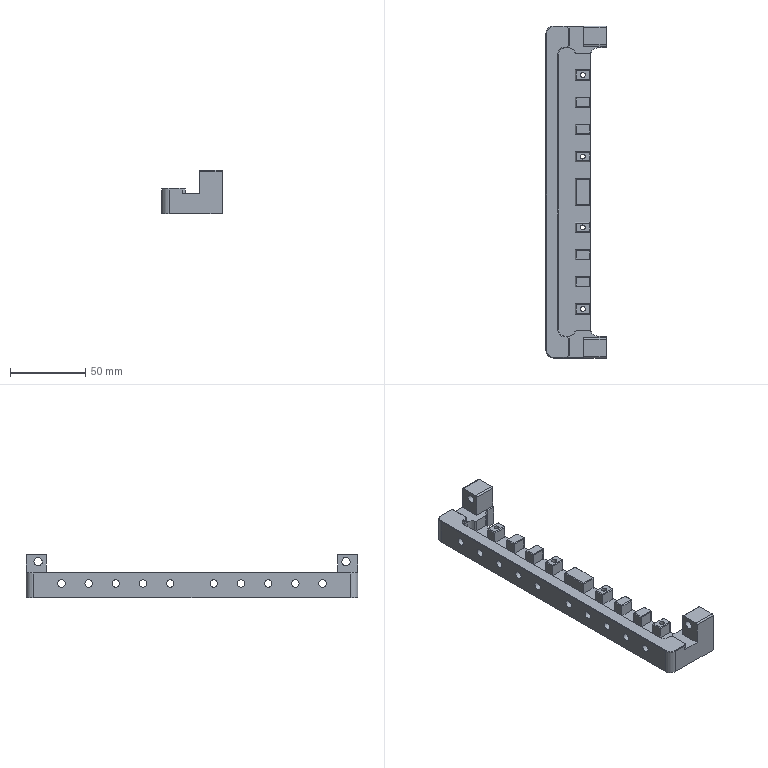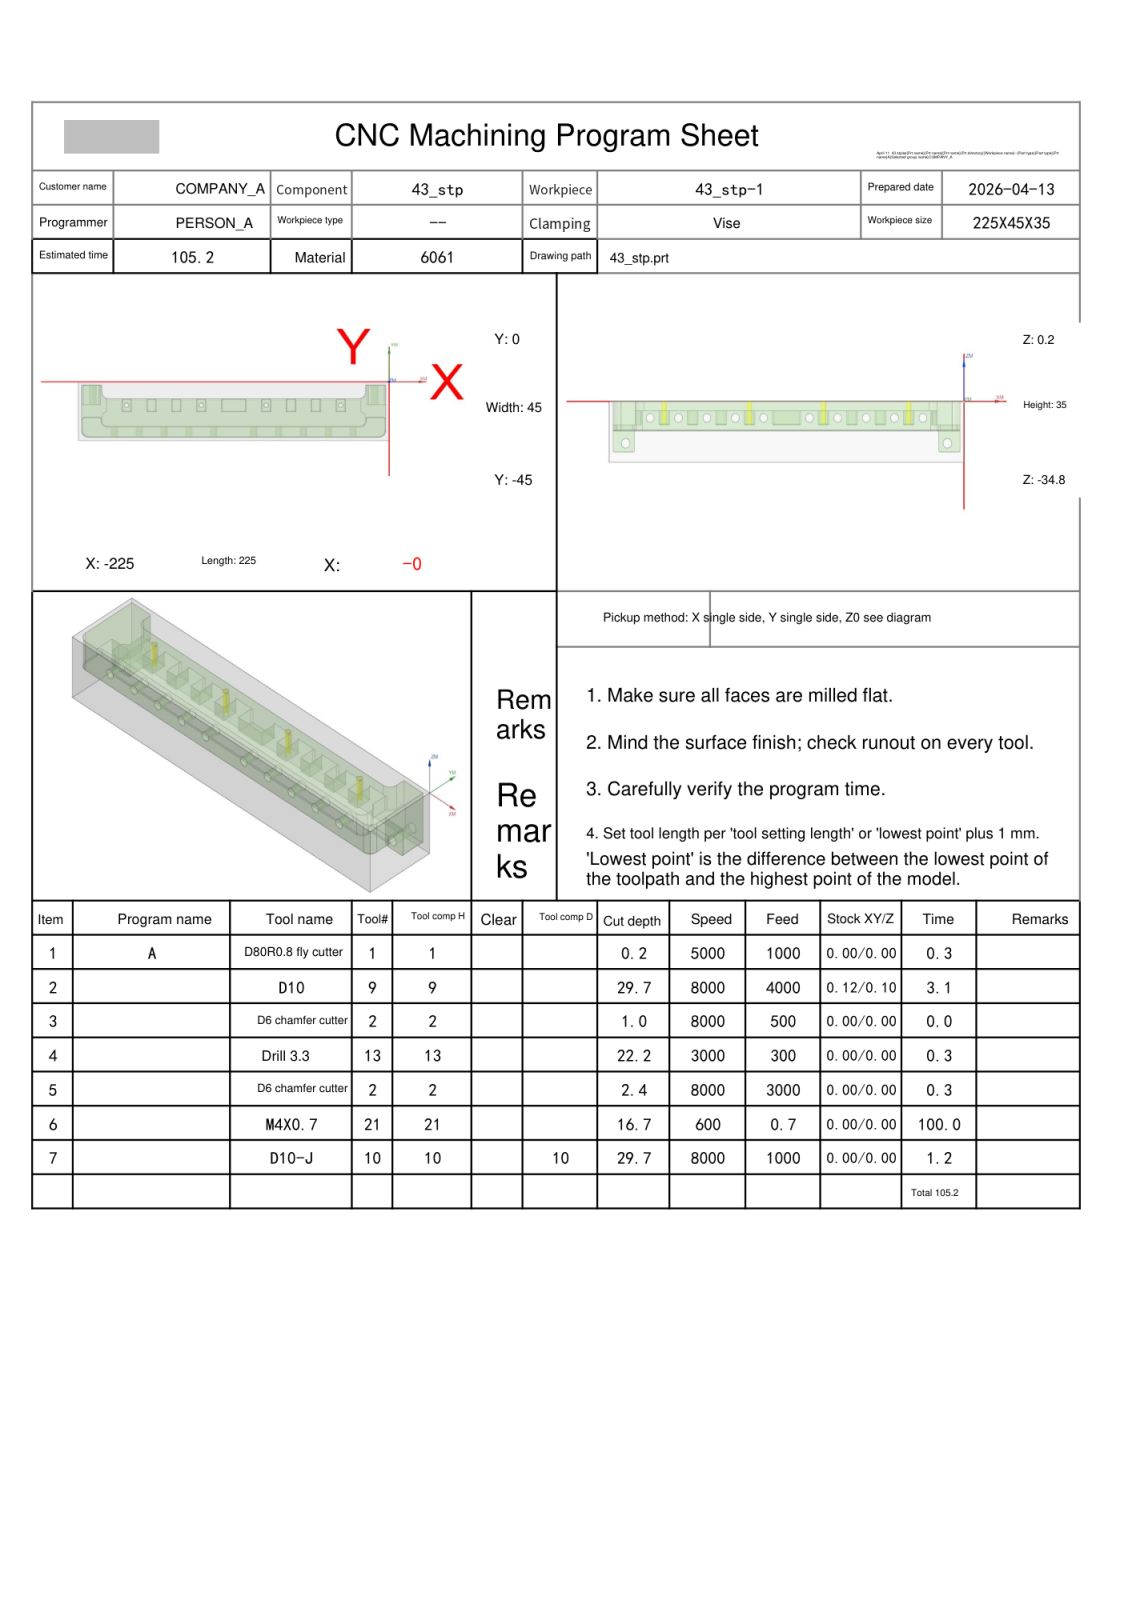NC program | NX | posted by the shop | part box 40 x 220 x 29 mm
Whole program:
%
O0001
(Machine time: 200.90 MIN)
(===Total Tool:6===)
(T1=D80R0.8 fly cutter D=80.  R=0.8  D-  H01 Z=0.    )
(T9=D10     D=10.  R=0.   D-  H09 Z=-29.5 )
(T2=D6 chamfer cutter   D=6.   R=0.   D-  H02 Z=-2.2  )
(T13=drill 3.3  D=3.3  DR_a=118 D-  H13 Z=-22.  )
(T21=M4X0.7 D=3.3  DR_a=180 D-  H21 Z=-16.5 )
(T10=D10-J  D=10.  R=0.   D10 H10 Z=-29.5 )
G80 G90 G17 G49 G40
G91 G28 Z0
M01
N1 T01 M06
(D80R0.8 fly cutter  D=80. R=0.8 H=01 ce=0.00 di=0.00)
G00 G90 G54 X-267.5 Y-22.5 M03 S5000
G43 H01 Z20.
M08
Z2.
G01 Z0.0 F1000.
X-262.5
X37.5
X42.5
Z2.
G00 Z20.
G91 G28 Z0.0
M05
M09
G91 G28 Z0.0
M01
N2 T09 M06
(D10  D=10. R=0. H=09 ce=0.12 di=0.10)
G00 G90 G54 X-223.344 Y10.981 M03 S8000
G43 H09 Z20.
M08
Z-12.75
G01 X-223.325 Y10.882 Z-13.375 F4000.
X-223.306 Y10.784 Z-13.622
X-223.288 Y10.686 Z-13.804
X-223.269 Y10.588 Z-13.95
X-223.25 Y10.489 Z-14.073
X-223.232 Y10.391 Z-14.178
X-223.213 Y10.293 Z-14.27
X-223.194 Y10.195 Z-14.35
X-223.176 Y10.096 Z-14.42
X-223.157 Y9.998 Z-14.482
X-223.138 Y9.9 Z-14.536
X-223.12 Y9.802 Z-14.583
X-223.101 Y9.703 Z-14.624
X-223.082 Y9.605 Z-14.658
X-223.064 Y9.507 Z-14.686
X-223.045 Y9.409 Z-14.71
X-223.026 Y9.311 Z-14.727
X-223.008 Y9.212 Z-14.74
X-222.989 Y9.114 Z-14.747
X-222.97 Y9.016 Z-14.75
X-222.569 Y6.902
G03 X-222.31 Y6.55 I.505 J.101
X-218.496 Y5.912 I4.013 J12.27
X-208.326 Y5.731 I10.17 J285.705
X-205.002 Y5.75 I0.0 J285.885
G01 X-1.882 Y5.733
G02 X4.2 Y1.629 I-.118 J-6.733
X5.522 Y-4.19 I-15.384 J-6.557
X5.77 Y-13.731 I-184.09 J-9.541
X5.749 Y-16.505 I-184.337 J0.0
G01 X5.724 Y-43.28
G02 X1.627 Y-49.201 I-6.717 J.27
X-4.033 Y-50.51 I-6.479 J15.125
X-12.653 Y-50.761 I-8.62 J147.776
X-14.667 Y-50.747 I0.0 J148.027
G01 X-223.127 Y-50.733
G02 X-229.068 Y-46.861 I.104 J6.655
X-230.511 Y-40.908 I14.588 J6.685
X-230.754 Y-32.801 I135.158 J8.107
X-230.745 Y-31.313 I135.401 J0.0
G01 X-230.732 Y-1.86
G02 X-226.099 Y4.373 I6.691 J-.136
X-221.457 Y5.073 I4.642 J-15.038
X-220.97 Y5.066 I0.0 J-15.738
G03 X-206.554 Y4.948 I14.417 J887.439
X-204.601 Y4.951 I0.0 J887.556
G01 X-3.742 Y4.928
G02 X2.732 Y.822 I-.382 J-7.759
X4.583 Y-5.588 I-14.424 J-7.638
X4.953 Y-14.439 I-105.636 J-8.85
X4.942 Y-15.977 I-106.006 J0.0
G01 X4.931 Y-41.197
G02 X.812 Y-47.738 I-7.768 J.325
X-5.52 Y-49.576 I-7.6 J14.357
X-14.483 Y-49.956 I-8.963 J105.453
X-16.149 Y-49.943 I0.0 J105.833
G01 X-221.297 Y-49.925
G02 X-227.708 Y-45.847 I.438 J7.766
X-229.569 Y-39.516 I14.23 J7.622
X-229.948 Y-30.971 I96.189 J8.545
X-229.939 Y-29.688 I96.568 J0.0
G01 X-229.929 Y-3.783
G02 X-225.735 Y2.582 I7.333 J-.267
X-220.029 Y4.001 I6.278 J-13.063
X-212.323 Y4.187 I7.706 J-159.524
X-209.156 Y4.155 I0.0 J-159.71
G01 X-5.662 Y4.128
G02 X-.368 Y2.123 I-.242 J-8.63
G01 X-.075 Y2.01
G02 X2.331 Y-.805 I-2.759 J-4.796
X3.908 Y-8.695 I-24.227 J-8.944
X4.167 Y-19.6 I-229.636 J-10.905
X4.148 Y-22.531 I-229.895 J0.0
X4.171 Y-29.172 I-942.737 J-6.641
X4.114 Y-39.55 I-942.76 J0.0
X-.751 Y-46.891 I-8.811 J.557
X-7.415 Y-48.748 I-8.141 J16.329
X-16.464 Y-49.146 I-9.049 J102.79
X-17.722 Y-49.138 I0.0 J103.188
G01 X-219.382 Y-49.124
G02 X-226.884 Y-44.248 I.409 J8.84
X-228.738 Y-37.655 I16.206 J8.114
X-229.142 Y-28.749 I98.095 J8.906
X-229.136 Y-27.668 I98.498 J0.0
G01 X-229.123 Y-5.608
G02 X-227.26 Y-.727 I8.05 J-.277
G01 X-226.934 Y.06
X-226.12 Y1.12
X-225.06 Y1.934
G02 X-221.782 Y2.835 I4.196 J-8.849
X-213.838 Y3.341 I7.945 J-62.222
X-213.084 Y3.336 I0.0 J-62.727
G01 X-7.582 Y3.331
G02 X-3.862 Y2.62 I-.386 J-12.102
X-3.247 Y2.636 I.615 J-11.741
X-1.25 Y2.465 I0.0 J-11.757
G01 X-.355 Y2.118
G03 X-2.498 Y2.62 I-2.3 J-4.994
G01 X-13.287 Y2.708
X-212.267 Y2.696
G02 X-220.3 Y2.614 I-8.033 J391.338
X-222.5 Y2.62 I0.0 J391.421
G01 X-223.825 Y2.446
X-222.5 Y2.62
X-208.499
G02 X-206.152 Y2.251 I-2.069 J-20.79
G03 X-198.832 Y1.909 I7.32 J78.288
X-197.466 Y1.921 I0.0 J78.63
G01 X-19.611 Y1.924
X-18.325 Y2.446
X-16.998 Y2.62
X-4.758
X-16.998
X-18.325 Y2.446
G02 X-22.587 Y1.431 I-4.372 J8.904
X-32.038 Y1.25 I-9.451 J247.294
X-35.239 Y1.271 I0.0 J247.474
G01 X-198.399 Y1.291
G02 X-199.141 Y1.286 I-.743 J60.472
X-205.411 Y1.612 I0.0 J60.477
G03 X-207.377 Y2.484 I-3.454 J-5.134
G02 X-205.244 Y1.488 I-1.568 J-6.142
G03 X-201.36 Y.711 I4.328 J11.54
X-192.699 Y.464 I8.661 J151.191
X-190.999 Y.473 I0.0 J151.439
G01 X-27.537 Y.497
G03 X-26.847 Y.491 I.689 J39.949
X-21.165 Y.897 I0.0 J39.955
X-20.62 Y1.12 I-.13 J1.093
G01 X-19.56 Y1.934
G02 X-20.933 Y.878 I-38.177 J48.225
X-24.61 Y.077 I-4.089 J9.927
X-32.322 Y-.168 I-7.712 J121.203
X-33.411 Y-.163 I0.0 J121.448
G01 X-194.159 Y-.149
G02 X-195.065 Y-.156 I-.906 J64.701
X-202.55 Y.279 I0.0 J64.707
X-204.506 Y.773 I1.363 J9.501
G03 X-205.486 Y1.629 I-5.241 J-5.016
G02 X-204.316 Y.595 I-7.173 J-9.304
G03 X-200.892 Y-.483 I4.249 J7.515
X-192.832 Y-.95 I8.06 J69.374
X-192.006 Y-.945 I0.0 J69.841
G01 X-31.763 Y-.95
G03 X-30.82 Y-.957 I.943 J58.104
X-23.627 Y-.511 I0.0 J58.112
X-21.402 Y.14 I-1.122 J7.971
G01 X-20.62 Y1.12
G02 X-21.586 Y-.042 I-5.634 J3.696
X-24.852 Y-1.12 I-4.103 J6.946
X-32.656 Y-1.592 I-7.803 J64.292
X-33.519 Y-1.586 I0.0 J64.764
G01 X-191.356 Y-1.587
G02 X-192.176 Y-1.591 I-.82 J71.795
X-200.337 Y-1.126 I0.0 J71.8
X-203.774 Y-.137 I1.104 J10.303
G01 X-204.502 Y.75
G03 X-203.457 Y-.461 I6.904 J4.905
X-199.935 Y-1.749 I4.686 J7.359
X-191.917 Y-2.353 I8.018 J52.913
G01 X-191.725 Y-2.352
X-181.241 Y-2.409
X-34.246 Y-2.388
G03 X-33.356 Y-2.394 I.89 J65.016
X-25.371 Y-1.902 I0.0 J65.022
X-21.831 Y-.719 I-.925 J8.659
X-21.434 Y.06 I-1.612 J1.312
G01 X-21.337 Y.187
G03 X-21.745 Y-.669 I4.324 J-2.589
G02 X-24.012 Y-1.985 I-3.415 J3.274
X-30.268 Y-2.884 I-6.746 J24.722
X-39.701 Y-3.051 I-9.433 J266.298
X-40.841 Y-3.048 I0.0 J266.465
G01 X-189.192 Y-3.022
G02 X-189.965 Y-3.026 I-.773 J74.208
X-198.8 Y-2.499 I0.0 J74.212
X-202.938 Y-1.237 I1.291 J11.653
X-203.561 Y-.449 I.454 J.999
G01 X-203.804 Y-.131
G02 X-203.329 Y-.995 I-1.964 J-1.643
G03 X-200.981 Y-2.502 I3.71 J3.199
X-194.703 Y-3.589 I7.204 J22.928
X-184.233 Y-3.856 I10.469 J205.08
X-182.279 Y-3.847 I0.0 J205.347
G01 X-36.485 Y-3.827
G03 X-35.636 Y-3.832 I.849 J73.825
X-26.938 Y-3.318 I0.0 J73.829
X-22.556 Y-1.916 I-1.175 J11.222
X-21.946 Y-1.175 I-.403 J.955
G01 X-21.701 Y-.584
G03 X-21.991 Y-1.444 I2.747 J-1.408
G02 X-23.905 Y-2.921 I-3.28 J2.273
X-29.579 Y-4.149 I-6.732 J17.374
X-39.66 Y-4.496 I-10.081 J146.179
X-41.487 Y-4.485 I0.0 J146.527
G01 X-186.162 Y-4.469
G02 X-187.141 Y-4.475 I-.979 J94.073
X-196.798 Y-3.978 I0.0 J94.078
X-201.925 Y-2.571 I1.403 J15.166
X-203.04 Y-1.712 I1.386 J2.95
G01 X-203.389 Y-.866
G03 X-202.718 Y-2.237 I4.509 J1.355
X-199.425 Y-4.037 I4.994 J5.224
X-191.828 Y-5.096 I8.376 J32.325
X-180.753 Y-5.295 I11.075 J307.788
X-178.681 Y-5.288 I0.0 J307.987
G01 X-38.881 Y-5.27
G03 X-37.914 Y-5.275 I.966 J86.627
X-28.491 Y-4.761 I0.0 J86.632
X-23.337 Y-3.24 I-1.362 J14.111
X-22.079 Y-2.106 I-1.406 J2.824
G01 X-21.966 Y-1.332
G02 X-22.185 Y-2.399 I-2.97 J.054
X-24.627 Y-4.237 I-4.171 J3.001
X-30.857 Y-5.566 I-7.471 J19.748
X-41.373 Y-5.935 I-10.517 J149.883
X-43.169 Y-5.924 I0.0 J150.251
G01 X-184.954 Y-5.902
G02 X-185.794 Y-5.906 I-.84 J88.947
X-195.95 Y-5.324 I0.0 J88.951
X-201.275 Y-3.795 I1.736 J16.076
X-202.949 Y-2.351 I1.816 J3.8
G01 X-203.053 Y-1.68
G03 X-201.925 Y-3.763 I2.566 J.042
X-197.428 Y-5.687 I6.53 J9.046
X-188.311 Y-6.611 I9.518 J48.494
X-176.856 Y-6.728 I11.456 J562.17
G01 X-176.201 Y-6.727
X-40.403 Y-6.706
G03 X-39.534 Y-6.711 I.869 J90.383
X-29.569 Y-6.16 I0.0 J90.387
X-23.912 Y-4.522 I-1.631 J16.227
X-22.15 Y-2.954 I-1.945 J3.959
G01 X-22.068 Y-2.102
X-22.13 Y-2.976
G02 X-23.925 Y-4.891 I-3.637 J1.612
X-29.548 Y-6.685 I-7.429 J13.568
X-39.318 Y-7.313 I-9.81 J76.328
G01 X-51.802 Y-7.367
X-182.802 Y-7.343
G02 X-183.68 Y-7.347 I-.877 J101.702
X-194.621 Y-6.756 I0.0 J101.706
X-200.666 Y-5.077 I1.856 J18.406
X-202.852 Y-3.177 I2.098 J4.62
G01 X-202.974 Y-2.288
G03 X-202.758 Y-3.553 I4.537 J.123
X-200.371 Y-5.734 I4.634 J2.674
X-194.367 Y-7.468 I8.136 J16.913
X-190.316 Y-7.88 I12.063 J98.418
G01 X-34.38 Y-7.868
G03 X-26.313 Y-6.623 I-.474 J29.843
X-22.512 Y-4.341 I-2.26 J8.07
X-22.12 Y-3.65 I-1.161 J1.115
G01 Y-2.85
G02 X-22.102 Y-3.212 I-3.689 J-.362
X-22.187 Y-4.002 I-3.706 J0.0
X-24.318 Y-6.161 I-4.367 J2.179
X-29.325 Y-7.88 I-7.486 J13.651
G01 X-34.765
G03 X-33.361 Y-7.882 I1.405 J548.197
X-27.689 Y-7.852 I0.0 J548.199
X-22.556 Y-5.331 I-.747 J8.007
X-22.12 Y-4.569 I-1.417 J1.316
G01 Y-3.689
G02 X-22.101 Y-4.086 I-4.259 J-.396
X-22.185 Y-4.925 I-4.277 J0.0
X-24.496 Y-7.243 I-4.469 J2.146
X-26.018 Y-7.88 I-4.271 J8.067
G01 X-28.098
G03 X-27.105 Y-7.899 I.993 J25.81
X-25.332 Y-7.838 I0.0 J25.829
X-22.157 Y-5.621 I-.875 J4.636
X-22.114 Y-4.861 I-6.739 J.761
X-22.12 Y-4.576 I-6.781 J0.0
G02 X-22.099 Y-4.981 I-3.882 J-.404
X-22.192 Y-5.827 I-3.903 J0.0
X-24.51 Y-7.88 I-3.51 J1.629
G01 X-25.71
G03 X-25.154 Y-7.9 I.556 J7.74
X-23.965 Y-7.808 I0.0 J7.76
X-22.134 Y-6.291 I-.741 J2.758
G01 X-22.12 Y-5.485
G02 X-22.101 Y-5.824 I-2.993 J-.339
X-22.193 Y-6.565 I-3.013 J0.0
X-23.633 Y-7.88 I-2.184 J.946
G01 X-24.353
G03 X-23.995 Y-7.904 I.358 J2.666
X-22.933 Y-7.686 I0.0 J2.69
X-22.12 Y-6.756 I-.602 J1.347
G01 Y-6.276
G02 X-22.097 Y-6.529 I-1.382 J-.253
X-23.116 Y-7.88 I-1.405 J0.0
G01 X-23.596
G03 X-23.333 Y-7.904 I.263 J1.421
X-22.2 Y-7.357 I0.0 J1.445
X-22.115 Y-6.917 I-1.088 J.44
G01 X-22.12 Y-6.806
G02 X-22.095 Y-7.012 I-.851 J-.206
X-22.971 Y-7.887 I-.876 J0.0
G01 X-23.085 Y-7.88
X-22.89 Y-7.905
G03 X-22.12 Y-7.134 I0.0 J.771
G01 Y-7.115
X-22.109 Y-7.231
G02 X-22.669 Y-7.869 I-.643 J0.0
G01 X-22.757 Y-7.876
G02 X-23.119 Y-7.724 I0.0 J.507
G01 X-23.97 Y-6.839
X-25.338 Y-5.419 Z-14.65
X-25.666 Y-5.078
X-25.715 Y-5.019
X-25.754 Y-4.954
X-25.782 Y-4.882
X-25.8 Y-4.808
X-25.806 Y-4.732
Y-1.289
X-25.799 Y-1.072
X-25.779 Y-.856
X-25.747 Y-.642
X-25.701 Y-.43
X-25.643 Y-.221
X-25.572 Y-.016
X-25.489 Y.184
X-25.394 Y.379
X-25.288 Y.568
X-25.17 Y.75
X-25.042 Y.925
X-24.903 Y1.091
X-24.754 Y1.249
X-21.449 Y4.555
X-21.292 Y4.702
X-21.126 Y4.84
X-20.952 Y4.967
X-20.771 Y5.084
X-20.583 Y5.189
X-20.389 Y5.282
X-20.189 Y5.363
X-19.985 Y5.432
X-19.777 Y5.489
X-19.566 Y5.532
X-19.353 Y5.563
X-18.74 Y5.623
X-18.126 Y5.669
X-17.511 Y5.7
X-16.896 Y5.716
X-.897 Y5.935
X-.665 Y5.932
X-.433 Y5.915
X-.203 Y5.885
X.025 Y5.843
X.251 Y5.787
X.473 Y5.719
X.691 Y5.638
X.903 Y5.545
X1.111 Y5.439
X1.311 Y5.323
X1.505 Y5.195
X1.692 Y5.056
X1.87 Y4.907
X3.479 Y3.481
X3.538 Y3.419
X3.586 Y3.348
X3.62 Y3.27
X3.641 Y3.187
X3.648 Y3.102
X3.64 Y3.017
X3.617 Y2.935
X3.377 Y2.278
X2.699 Y.427 Z-14.75
X2.331 Y-.594
G03 X2.599 Y-2.038 I8.053 J.75
X3.054 Y-8.352 I160.008 J8.355
G02 X3.358 Y-20.581 I-245.675 J-12.228
X3.346 Y-23.067 I-245.979 J0.0
X3.369 Y-28.689 I-682.247 J-5.622
X3.307 Y-37.846 I-682.27 J0.0
X-1.88 Y-45.916 I-9.586 J.46
G01 X-3.63 Y-46.85
G02 X-9.882 Y-48.04 I-7.448 J22.123
X-20.208 Y-48.354 I-10.326 J169.331
X-22.195 Y-48.343 I0.0 J169.646
G01 X-217.535 Y-48.323
G02 X-225.903 Y-43.139 I.191 J9.654
G01 X-226.845 Y-41.384
G02 X-228.032 Y-35.205 I21.82 J7.397
X-228.356 Y-24.788 I167.496 J10.417
X-228.343 Y-22.732 I167.819 J0.0
X-228.365 Y-16.599 I837.721 J6.134
X-228.314 Y-7.313 I837.743 J0.0
X-227.62 Y-4.001 I12.209 J-.83
X-227.641 Y-3.302 I11.67 J.699
X-227.446 Y-1.175 I11.691 J0.0
G01 X-227.231 Y-.657
X-227.446 Y-1.175
G03 X-227.641 Y-3.302 I11.496 J-2.127
X-227.62 Y-4.001 I11.691 J0.0
X-227.717 Y-17.092 I880.272 J-13.091
X-227.62 Y-30.172 I880.37 J0.0
G01 Y-37.499
X-227.424 Y-39.479
X-227.62 Y-37.499
Y-4.812
G03 X-228.12 Y-4.312 I-.5 J0.0
X-228.533 Y-4.531 I0.0 J-.5
G01 X-228.967 Y-5.167
X-230.077 Y-6.797 Z-14.65
X-230.67 Y-7.668
X-230.707 Y-7.732
X-230.735 Y-7.802
X-230.751 Y-7.875
X-230.757 Y-7.949
Y-35.257
X-230.751 Y-35.904
X-230.732 Y-36.551
X-230.702 Y-37.197
X-230.66 Y-37.843
X-230.605 Y-38.488
X-230.538 Y-39.131
X-230.459 Y-39.774
X-230.162 Y-42.022
X-230.145 Y-42.101
X-230.116 Y-42.176
X-230.075 Y-42.245
X-230.024 Y-42.307
X-229.963 Y-42.36
X-229.895 Y-42.402
X-229.82 Y-42.433
X-229.742 Y-42.451
X-229.033 Y-42.56
X-227.084 Y-42.857 Z-14.75
X-226.116 Y-43.011
X-225.877 Y-43.171
X-224.636 Y-44.676
X-223.093 Y-45.934
X-221.333 Y-46.866
X-219.482 Y-47.427
G03 X-214.513 Y-47.701 I4.969 J44.773
X-213.557 Y-47.691 I0.0 J45.048
G01 X-18.778 Y-47.684
G02 X-9.908 Y-47.615 I8.87 J-571.75
X-7.501 Y-47.62 I0.0 J-571.818
G01 X-5.528 Y-47.426
X-7.501 Y-47.62
X-217.557
G03 X-217.958 Y-47.821 I.004 J-.509
G01 X-218.326 Y-48.316
X-219.503 Y-49.898 Z-14.65
X-220.042 Y-50.623
X-220.095 Y-50.683
X-220.158 Y-50.735
X-220.228 Y-50.775
X-220.303 Y-50.804
X-220.382 Y-50.82
X-220.463 Y-50.824
X-220.543 Y-50.814
X-220.621 Y-50.792
X-220.694 Y-50.757
X-228.019 Y-46.516
X-228.201 Y-46.401
X-228.375 Y-46.275
X-228.539 Y-46.136
X-228.693 Y-45.986
X-228.836 Y-45.825
X-228.967 Y-45.655
X-229.086 Y-45.476
X-229.192 Y-45.289
X-229.285 Y-45.095
X-229.363 Y-44.895
X-229.427 Y-44.69
X-229.477 Y-44.481
X-229.933 Y-42.202
X-230.071 Y-41.478
X-230.197 Y-40.751
X-230.31 Y-40.022
X-230.411 Y-39.292
X-230.5 Y-38.56
X-230.576 Y-37.826
X-230.639 Y-37.091
X-230.689 Y-36.355
X-230.727 Y-35.619
X-230.752 Y-34.881
X-231.358 Y-11.255
X-231.373 Y-10.402
X-231.372 Y-9.548
X-231.357 Y-8.695
X-231.327 Y-7.841
X-231.282 Y-6.989
X-231.223 Y-6.137
X-231.148 Y-5.287
X-231.059 Y-4.438
X-230.956 Y-3.591
X-230.837 Y-2.745
X-230.704 Y-1.902
X-230.144 Y1.457
X-230.103 Y1.656
X-230.048 Y1.851
X-229.978 Y2.041
X-229.894 Y2.226
X-229.797 Y2.404
X-229.687 Y2.574
X-229.565 Y2.735
X-229.431 Y2.887
X-229.286 Y3.029
X-229.131 Y3.159
X-228.966 Y3.278
X-228.794 Y3.384
X-226.274 Y4.804
X-225.971 Y4.968
X-225.661 Y5.119
X-225.345 Y5.258
X-225.025 Y5.384
X-224.699 Y5.498
X-224.369 Y5.598
X-224.036 Y5.686
X-223.699 Y5.76
X-223.36 Y5.821
X-223.019 Y5.869
X-222.676 Y5.903
X-222.331 Y5.923
X-221.987 Y5.93
X-205.811
X-205.618 Y5.923
X-205.427 Y5.9
X-205.237 Y5.863
X-205.051 Y5.811
X-204.87 Y5.745
X-204.694 Y5.666
X-204.524 Y5.572
X-204.363 Y5.466
X-204.21 Y5.348
X-204.067 Y5.219
X-203.934 Y5.078
X-203.813 Y4.928
X-200.662 Y.712
X-200.62 Y.645
X-200.589 Y.572
X-200.569 Y.495
X-200.562 Y.417
X-200.568 Y.338
X-200.586 Y.261
X-200.616 Y.188
X-200.657 Y.12
X-200.932 Y-.263
X-202.084 Y-1.863 Z-14.75
X-202.826 Y-2.905
G03 X-202.862 Y-3.272 I1.883 J-.367
X-202.365 Y-4.56 I1.919 J0.0
X-198.858 Y-6.975 I6.093 J5.095
X-195.767 Y-7.88 I8.008 J21.612
G01 X-190.247
G02 X-192.537 Y-7.891 I-2.29 J239.621
X-196.938 Y-7.851 I0.0 J239.632
X-202.342 Y-5.132 I.847 J8.414
X-202.88 Y-4.176 I2.127 J1.825
G01 Y-3.296
G03 X-202.905 Y-3.727 I3.715 J-.431
X-202.721 Y-4.885 I3.74 J0.0
X-199.931 Y-7.475 I5.146 J2.747
G01 X-198.938 Y-7.88
X-196.538
X-199.292 Y-7.86
G02 X-202.861 Y-5.195 I.869 J4.886
G01 X-202.88 Y-4.293
G03 X-202.903 Y-4.691 I3.42 J-.398
X-202.722 Y-5.794 I3.443 J0.0
X-200.432 Y-7.88 I3.692 J1.753
G01 X-199.072
G02 X-199.66 Y-7.898 I-.588 J9.408
X-200.796 Y-7.83 I0.0 J9.426
X-202.88 Y-5.91 I.806 J2.966
G01 Y-5.19
G03 X-202.903 Y-5.556 I2.834 J-.366
X-202.698 Y-6.621 I2.857 J0.0
X-201.311 Y-7.88 I2.138 J.961
G01 X-200.511
G02 X-200.881 Y-7.9 I-.37 J3.47
X-201.678 Y-7.807 I0.0 J3.49
X-202.88 Y-6.549 I.677 J1.85
G01 Y-6.069
G03 X-202.904 Y-6.35 I1.632 J-.281
X-201.906 Y-7.87 I1.656 J0.0
G01 X-201.369 Y-7.88
G02 X-201.62 Y-7.904 I-.251 J1.31
X-202.873 Y-7.027 I0.0 J1.334
G01 X-202.88 Y-6.588
G03 X-202.902 Y-6.817 I1.178 J-.228
X-202.329 Y-7.84 I1.2 J0.0
X-201.881 Y-7.88 I.507 J3.147
G01 X-202.076 Y-7.904
G02 X-202.882 Y-7.097 I0.0 J.807
G01 X-202.88 Y-7.035
X-202.9 Y-7.2
G03 X-202.22 Y-7.88 I.681 J0.0
G01 X-202.195
G03 X-201.741 Y-7.596 I-.002 J.509
G01 X-200.82 Y-5.7
G02 X-200.378 Y-5.415 I.457 J-.225
G01 X-200.278 Y-5.413 Z-14.747
X-200.178 Y-5.41 Z-14.74
X-200.078 Y-5.408 Z-14.727
X-199.978 Y-5.405 Z-14.71
X-199.878 Y-5.403 Z-14.686
X-199.778 Y-5.4 Z-14.658
X-199.678 Y-5.398 Z-14.624
X-199.578 Y-5.396 Z-14.583
X-199.478 Y-5.393 Z-14.536
X-199.378 Y-5.391 Z-14.482
X-199.278 Y-5.388 Z-14.42
X-199.178 Y-5.386 Z-14.35
X-199.078 Y-5.383 Z-14.27
X-198.978 Y-5.381 Z-14.178
X-198.878 Y-5.378 Z-14.073
X-198.778 Y-5.376 Z-13.95
X-198.678 Y-5.373 Z-13.804
X-198.578 Y-5.371 Z-13.622
X-198.478 Y-5.368 Z-13.375
X-198.378 Y-5.366 Z-12.75
G00 Z20.
X5.258 Y-3.841
Z-12.75
G01 X5.247 Y-3.742 Z-13.375
X5.237 Y-3.642 Z-13.622
X5.226 Y-3.543 Z-13.804
X5.215 Y-3.443 Z-13.95
X5.204 Y-3.344 Z-14.073
X5.194 Y-3.245 Z-14.178
X5.183 Y-3.145 Z-14.27
X5.172 Y-3.046 Z-14.35
X5.162 Y-2.946 Z-14.42
X5.151 Y-2.847 Z-14.482
X5.14 Y-2.747 Z-14.536
X5.13 Y-2.648 Z-14.583
X5.119 Y-2.549 Z-14.624
X5.108 Y-2.449 Z-14.658
X5.097 Y-2.35 Z-14.686
X5.087 Y-2.25 Z-14.71
X5.076 Y-2.151 Z-14.727
X5.065 Y-2.051 Z-14.74
X5.055 Y-1.952 Z-14.747
X5.044 Y-1.853 Z-14.75
G03 X4.542 Y-1.402 I-.502 J-.054
X4.274 Y-1.479 I0.0 J-.505
G01 X2.857 Y-2.367
G03 X2.62 Y-2.795 I.274 J-.431
G01 Y-37.501
X2.425 Y-39.477
X1.849 Y-41.375
X.913 Y-43.124
X-.346 Y-44.657
X-1.88 Y-45.916
G03 X-2.064 Y-46.307 I.323 J-.391
X-2.025 Y-46.503 I.507 J0.0
G01 X-1.235 Y-48.366
X-1.196 Y-48.458 Z-14.747
X-1.157 Y-48.55 Z-14.74
X-1.118 Y-48.642 Z-14.727
X-1.079 Y-48.734 Z-14.71
X-1.04 Y-48.826 Z-14.686
X-1.001 Y-48.918 Z-14.658
X-.962 Y-49.01 Z-14.624
X-.923 Y-49.102 Z-14.583
X-.884 Y-49.194 Z-14.536
X-.845 Y-49.286 Z-14.482
X-.806 Y-49.378 Z-14.42
X-.767 Y-49.47 Z-14.35
X-.728 Y-49.563 Z-14.27
X-.689 Y-49.655 Z-14.178
X-.65 Y-49.747 Z-14.073
X-.611 Y-49.839 Z-13.95
X-.572 Y-49.931 Z-13.804
X-.533 Y-50.023 Z-13.622
X-.494 Y-50.115 Z-13.375
X-.455 Y-50.207 Z-12.75
G00 Z20.
X-223.524 Y10.93
Z-27.5
G01 X-223.505 Y10.832 Z-28.125
X-223.487 Y10.734 Z-28.372
X-223.468 Y10.636 Z-28.554
X-223.449 Y10.538 Z-28.7
X-223.43 Y10.439 Z-28.823
X-223.412 Y10.341 Z-28.928
X-223.393 Y10.243 Z-29.02
X-223.374 Y10.145 Z-29.1
X-223.356 Y10.046 Z-29.17
X-223.337 Y9.948 Z-29.232
X-223.318 Y9.85 Z-29.286
X-223.3 Y9.752 Z-29.333
X-223.281 Y9.653 Z-29.374
X-223.262 Y9.555 Z-29.408
X-223.243 Y9.457 Z-29.436
X-223.225 Y9.359 Z-29.46
X-223.206 Y9.26 Z-29.477
X-223.187 Y9.162 Z-29.49
X-223.169 Y9.064 Z-29.497
X-223.15 Y8.966 Z-29.5
X-222.747 Y6.851
G03 X-222.489 Y6.5 I.505 J.101
X-218.685 Y5.862 I4.013 J12.278
X-209.467 Y5.687 I9.217 J242.485
X-206.951 Y5.7 I0.0 J242.66
G01 X-1.752 Y5.676
G02 X4.025 Y1.811 I-.243 J-6.612
X5.461 Y-4.139 I-14.623 J-6.679
X5.703 Y-12.252 I-135.861 J-8.113
X5.695 Y-13.734 I-136.104 J0.0
G01 X5.676 Y-43.25
G02 X1.811 Y-49.025 I-6.611 J.244
X-4.139 Y-50.461 I-6.676 J14.611
X-12.252 Y-50.703 I-8.112 J135.794
X-13.734 Y-50.695 I0.0 J136.036
G01 X-223.25 Y-50.676
G02 X-229.025 Y-46.811 I.244 J6.611
X-230.461 Y-40.861 I14.611 J6.676
X-230.703 Y-32.748 I135.794 J8.112
X-230.695 Y-31.266 I136.036 J0.0
G01 X-230.676 Y-1.75
G02 X-225.919 Y4.356 I6.608 J-.243
X-221.267 Y5.006 I4.653 J-16.324
X-220.78 Y4.999 I0.0 J-16.975
G03 X-207.357 Y4.897 I13.423 J889.352
X-204.952 Y4.901 I0.0 J889.453
G01 X-3.852 Y4.883
G02 X2.648 Y.821 I-.326 J-7.754
X4.498 Y-5.349 I-13.99 J-7.555
X4.896 Y-13.868 I-90.778 J-8.518
X4.888 Y-15.096 I-91.177 J0.0
G01 X4.881 Y-41.167
G02 X.852 Y-47.629 I-7.744 J.342
X-5.233 Y-49.483 I-7.517 J13.763
X-13.951 Y-49.9 I-8.718 J90.831
X-15.379 Y-49.889 I0.0 J91.249
G01 X-221.167 Y-49.881
G02 X-227.629 Y-45.852 I.342 J7.744
X-229.483 Y-39.767 I13.763 J7.517
X-229.9 Y-31.049 I90.831 J8.718
X-229.889 Y-29.621 I91.249 J0.0
G01 X-229.881 Y-3.833
G02 X-225.829 Y2.45 I7.313 J-.269
X-219.658 Y3.961 I6.689 J-13.964
X-212.044 Y4.13 I7.613 J-171.09
X-209.028 Y4.103 I0.0 J-171.259
G01 X-5.851 Y4.085
G02 X-.609 Y2.216 I-.119 J-8.623
G01 X-.068 Y2.006
G02 X2.338 Y-.824 I-2.769 J-4.792
X3.888 Y-9.13 I-26.42 J-9.227
X4.11 Y-19.504 I-242.254 J-10.374
X4.098 Y-21.927 I-242.476 J0.0
X4.123 Y-28.883 I-969.388 J-6.956
X4.064 Y-39.506 I-969.413 J0.0
X-.739 Y-46.803 I-8.805 J.567
X-7.561 Y-48.709 I-8.227 J16.284
X-17.093 Y-49.105 I-9.532 J114.697
X-18.83 Y-49.091 I0.0 J115.092
G01 X-219.13 Y-49.084
G02 X-226.805 Y-44.258 I.199 J8.832
X-228.709 Y-37.439 I16.282 J8.223
X-229.105 Y-27.907 I114.689 J9.532
X-229.091 Y-26.17 I115.085 J0.0
G01 X-229.084 Y-5.871
G02 X-227.371 Y-.994 I8.036 J-.084
G01 X-226.934 Y.06
X-226.12 Y1.12
X-225.06 Y1.934
G02 X-222.251 Y2.733 I3.542 J-7.11
X-213.824 Y3.289 I8.428 J-63.648
X-212.996 Y3.284 I0.0 J-64.204
G01 X-7.612 Y3.28
G02 X-4.044 Y2.62 I-.436 J-12.323
X-3.329 Y2.64 I.714 J-12.372
X-1.246 Y2.464 I0.0 J-12.393
G01 X-.575 Y2.203
X-1.246 Y2.464
G03 X-3.329 Y2.64 I-2.084 J-12.217
X-4.044 Y2.62 I0.0 J-12.393
G02 X-10.459 Y2.598 I-6.416 J931.399
X-20.838 Y2.656 I0.0 J931.421
G01 X-212.218 Y2.644
X-222.5 Y2.62
X-223.825 Y2.446
X-222.5 Y2.62
X-208.499
G02 X-206.374 Y2.258 I-1.044 J-12.567
G03 X-200.148 Y1.886 I6.225 J51.785
X-199.548 Y1.889 I0.0 J52.158
G01 X-190.312 Y1.861
X-19.772 Y1.855
X-18.325 Y2.446
X-16.998 Y2.62
X-18.325 Y2.446
G02 X-20.286 Y1.671 I-6.297 J13.074
X-25.373 Y1.259 I-5.087 J31.185
X-25.825 Y1.262 I0.0 J31.597
G01 X-36.309 Y1.221
X-198.662 Y1.245
G02 X-199.436 Y1.239 I-.774 J50.969
X-205.394 Y1.588 I0.0 J50.975
G03 X-207.223 Y2.437 I-3.085 J-4.254
G02 X-205.37 Y1.545 I-1.043 J-4.537
G03 X-202.07 Y.737 I3.83 J8.509
X-194.211 Y.425 I7.859 J98.663
X-193.096 Y.431 I0.0 J98.976
G01 X-28.038 Y.441
G03 X-27.237 Y.434 I.801 J45.313
X-21.383 Y.814 I0.0 J45.32
X-20.62 Y1.12 I-.024 J1.162
G01 X-19.56 Y1.934
X-20.938 Y.848
G02 X-24.435 Y.047 I-3.951 J9.216
X-32.382 Y-.222 I-7.947 J117.172
X-33.759 Y-.214 I0.0 J117.441
G01 X-194.109 Y-.199
G02 X-195.028 Y-.205 I-.92 J63.798
X-202.493 Y.233 I0.0 J63.804
X-204.533 Y.781 I.537 J6.069
G03 X-205.485 Y1.628 I-4.119 J-3.672
G02 X-204.277 Y.554 I-7.297 J-9.428
G03 X-200.841 Y-.531 I4.263 J7.52
X-193.029 Y-.992 I7.812 J65.959
X-192.428 Y-.989 I0.0 J66.42
G01 X-184.631 Y-1.018
X-31.715 Y-1.
G03 X-30.846 Y-1.006 I.868 J58.468
X-23.725 Y-.571 I0.0 J58.474
X-21.391 Y.13 I-.676 J6.486
G01 X-20.672 Y1.053
G02 X-21.622 Y-.091 I-5.643 J3.718
X-24.884 Y-1.169 I-4.099 J6.928
X-32.68 Y-1.642 I-7.796 J64.072
X-33.548 Y-1.636 I0.0 J64.545
G01 X-190.99 Y-1.639
G02 X-191.885 Y-1.644 I-.895 J76.01
X-200.149 Y-1.193 I0.0 J76.016
X-203.73 Y-.184 I1.08 J10.689
G01 X-204.446 Y.69
G03 X-203.285 Y-.604 I4.892 J3.219
X-199.298 Y-1.898 I5.067 J8.824
X-190.742 Y-2.429 I8.555 J68.662
X-190.106 Y-2.426 I0.0 J69.193
G01 X-182.952 Y-2.459
X-34.118 Y-2.436
G03 X-33.362 Y-2.44 I.756 J65.694
X-25.539 Y-1.973 I0.0 J65.699
X-21.905 Y-.798 I-.947 J9.138
X-21.434 Y.06 I-1.37 J1.309
G01 X-21.385 Y.123
X-21.759 Y-.703
G02 X-24.094 Y-2.051 I-3.465 J3.305
X-30.448 Y-2.941 I-6.803 J25.441
X-40.627 Y-3.107 I-10.179 J313.243
X-42.952 Y-3.098 I0.0 J313.408
G01 X-189.063 Y-3.072
G02 X-189.873 Y-3.077 I-.81 J74.64
X-198.75 Y-2.547 I0.0 J74.645
X-203.047 Y-1.191 I1.168 J11.187
X-203.562 Y-.447 I.58 J.951
G01 X-203.757 Y-.193
G02 X-203.321 Y-1.018 I-2.04 J-1.605
G03 X-200.937 Y-2.551 I3.752 J3.214
X-194.653 Y-3.638 I7.217 J23.015
X-184.169 Y-3.906 I10.483 J205.516
X-182.229 Y-3.896 I0.0 J205.783
G01 X-36.831 Y-3.879
G03 X-35.96 Y-3.884 I.871 J80.121
X-27.273 Y-3.412 I0.0 J80.126
X-22.744 Y-2.065 I-1.177 J12.252
X-21.965 Y-1.323 I-.587 J1.395
G02 X-21.701 Y-.584 I3.888 J-.974
G03 X-21.997 Y-1.479 I2.659 J-1.378
G02 X-24.029 Y-3.013 I-3.38 J2.365
X-29.826 Y-4.219 I-6.804 J18.173
X-40.455 Y-4.553 I-10.629 J168.624
X-42.792 Y-4.537 I0.0 J168.959
G01 X-186.033 Y-4.52
G02 X-187.047 Y-4.525 I-1.013 J94.775
X-196.748 Y-4.027 I0.0 J94.78
X-201.826 Y-2.654 I1.465 J15.492
X-203.017 Y-1.764 I1.493 J3.241
G01 X-203.381 Y-.885
G03 X-202.808 Y-2.153 I5.618 J1.776
X-199.957 Y-3.9 I4.61 J4.322
X-193.135 Y-5.064 I7.937 J25.965
X-182.352 Y-5.343 I10.783 J207.909
X-180.548 Y-5.335 I0.0 J208.188
G01 X-38.278 Y-5.313
G03 X-37.549 Y-5.317 I.729 J80.191
X-28.35 Y-4.787 I0.0 J80.195
X-23.359 Y-3.29 I-1.458 J13.925
X-22.097 Y-2.181 I-1.685 J3.189
G01 X-21.961 Y-1.29
G02 X-22.192 Y-2.44 I-3.194 J.044
X-24.601 Y-4.266 I-4.175 J3.006
X-30.886 Y-5.616 I-7.503 J19.62
X-41.404 Y-5.984 I-10.518 J150.123
X-43.198 Y-5.974 I0.0 J150.491
G01 X-184.112 Y-5.959
G02 X-185.145 Y-5.964 I-1.033 J100.677
X-195.47 Y-5.433 I0.0 J100.682
X-201.059 Y-3.941 I1.684 J17.518
X-202.952 Y-2.365 I1.691 J3.956
G01 X-203.053 Y-1.679
G03 X-201.933 Y-3.786 I2.589 J.025
X-197.447 Y-5.723 I6.533 J8.963
X-188.493 Y-6.653 I9.436 J47.319
X-177.832 Y-6.777 I11.523 J531.12
G01 X-40.275 Y-6.755
G03 X-39.486 Y-6.758 I.79 J89.424
X-29.593 Y-6.209 I0.0 J89.428
X-23.928 Y-4.57 I-1.629 J16.238
X-22.162 Y-3.021 I-2.141 J4.223
G01 X-22.068 Y-2.102
X-22.13 Y-3.006
G02 X-23.854 Y-4.887 I-3.57 J1.541
X-29.369 Y-6.703 I-7.356 J13.056
X-39.45 Y-7.373 I-10.081 J75.541
G01 X-39.815 Y-7.372
X-50.072 Y-7.416
X-181.802 Y-7.4
G02 X-182.993 Y-7.406 I-1.191 J113.265
X-194.356 Y-6.834 I0.0 J113.271
X-200.446 Y-5.225 I1.88 J19.439
X-202.845 Y-3.222 I2.134 J4.995
G01 X-202.963 Y-2.367
G03 X-202.754 Y-3.586 I4.335 J.116
X-200.382 Y-5.762 I4.645 J2.684
X-194.321 Y-7.517 I8.156 J16.828
X-190.971 Y-7.88 I26.348 J227.264
G01 X-33.838 Y-7.867
G03 X-25.946 Y-6.538 I-.492 J27.023
X-22.494 Y-4.359 I-2.395 J7.614
X-22.12 Y-3.681 I-1.141 J1.073
G01 Y-2.881
G02 X-22.101 Y-3.249 I-3.571 J-.368
X-22.19 Y-4.045 I-3.59 J0.0
X-24.482 Y-6.299 I-4.51 J2.292
X-29.105 Y-7.88 I-7.306 J13.814
G01 X-34.225
G03 X-31.706 Y-7.899 I2.519 J169.014
X-27.514 Y-7.847 I0.0 J169.032
X-22.561 Y-5.374 I-.821 J7.841
X-22.12 Y-4.607 I-1.43 J1.332
G01 Y-3.727
G02 X-22.101 Y-4.124 I-4.166 J-.397
X-22.187 Y-4.967 I-4.185 J0.0
X-24.512 Y-7.283 I-4.441 J2.133
X-25.927 Y-7.88 I-4.752 J9.282
G01 X-27.927
G03 X-26.928 Y-7.905 I.999 J20.012
X-25.242 Y-7.834 I0.0 J20.037
X-22.156 Y-5.654 I-.895 J4.541
X-22.115 Y-4.875 I-7.427 J.779
X-22.12 Y-4.61 I-7.468 J0.0
G02 X-22.101 Y-5.008 I-4.195 J-.398
X-22.185 Y-5.847 I-4.214 J0.0
X-24.47 Y-7.88 I-3.442 J1.567
G01 X-25.67
G03 X-25.113 Y-7.9 I.557 J7.624
X-23.924 Y-7.807 I0.0 J7.644
X-22.141 Y-6.347 I-.809 J2.807
G01 X-22.12 Y-5.521
G02 X-22.101 Y-5.856 I-2.93 J-.336
X-22.196 Y-6.599 I-2.949 J0.0
X-23.615 Y-7.88 I-2.143 J.947
G01 X-24.335
G03 X-23.973 Y-7.904 I.362 J2.702
X-22.935 Y-7.699 I0.0 J2.726
X-22.12 Y-6.767 I-.57 J1.321
G01 Y-6.287
G02 X-22.097 Y-6.541 I-1.372 J-.255
X-23.098 Y-7.88 I-1.395 J0.0
G01 X-23.578
G03 X-23.315 Y-7.904 I.263 J1.404
X-22.204 Y-7.374 I0.0 J1.429
X-22.114 Y-6.934 I-1.034 J.44
G01 X-22.12 Y-6.819
G02 X-22.096 Y-7.023 I-.841 J-.204
X-22.961 Y-7.889 I-.865 J0.0
G01 X-23.085 Y-7.88
X-22.891 Y-7.904
G03 X-22.12 Y-7.277 I0.0 J.787
G01 Y-7.117
X-22.11 Y-7.231
G02 X-22.587 Y-7.852 I-.643 J0.0
G01 X-22.685 Y-7.862
G02 X-23.048 Y-7.708 I0.0 J.506
G01 X-23.878 Y-6.843
X-25.242 Y-5.419 Z-29.4
X-25.585 Y-5.061
X-25.634 Y-5.002
X-25.673 Y-4.937
X-25.701 Y-4.866
X-25.718 Y-4.791
X-25.724 Y-4.715
Y-1.273
X-25.718 Y-1.056
X-25.698 Y-.84
X-25.665 Y-.626
X-25.62 Y-.414
X-25.562 Y-.205
X-25.491 Y0.0
X-25.408 Y.2
X-25.313 Y.395
X-25.207 Y.584
X-25.089 Y.766
X-24.96 Y.941
X-24.821 Y1.107
X-24.673 Y1.265
X-21.367 Y4.571
X-21.21 Y4.718
X-21.045 Y4.856
X-20.871 Y4.984
X-20.689 Y5.1
X-20.501 Y5.205
X-20.307 Y5.298
X-20.108 Y5.38
X-19.904 Y5.449
X-19.696 Y5.505
X-19.484 Y5.548
X-19.271 Y5.579
X-18.659 Y5.64
X-18.045 Y5.685
X-17.43 Y5.716
X-16.814 Y5.731
X-.812 Y5.931
X-.584 Y5.927
X-.356 Y5.91
X-.13 Y5.88
X.095 Y5.837
X.316 Y5.781
X.534 Y5.713
X.748 Y5.632
X.956 Y5.539
X1.159 Y5.434
X1.355 Y5.317
X1.545 Y5.189
X1.727 Y5.051
X1.9 Y4.902
X3.486 Y3.461
X3.544 Y3.399
X3.59 Y3.329
X3.624 Y3.251
X3.644 Y3.169
X3.65 Y3.085
X3.642 Y3.001
X3.62 Y2.92
X3.383 Y2.27
X2.709 Y.417 Z-29.5
X2.338 Y-.616
G03 X2.601 Y-2.062 I6.344 J.407
X3.035 Y-8.749 I153.009 J6.565
G02 X3.305 Y-20.726 I-265.238 J-11.977
X3.295 Y-22.985 I-265.508 J0.0
X3.315 Y-28.623 I-794.602 J-5.639
X3.264 Y-37.684 I-794.622 J0.0
X-1.524 Y-45.624 I-9.495 J.312
G01 X-1.88 Y-45.916
X-3.63 Y-46.85
G02 X-9.091 Y-47.931 I-6.693 J19.487
X-19.361 Y-48.3 I-10.27 J142.701
X-21.082 Y-48.29 I0.0 J143.07
G01 X-217.382 Y-48.278
G02 X-225.619 Y-43.484 I.032 J9.528
G01 X-225.902 Y-43.14
X-226.844 Y-41.385
G02 X-227.93 Y-35.917 I19.401 J6.694
X-228.292 Y-26.146 I131.83 J9.771
X-228.286 Y-24.886 I132.192 J0.0
X-228.318 Y-17.361 I881.765 J7.525
X-228.261 Y-7.307 I881.797 J0.0
X-227.62 Y-4.167 I12.829 J-.983
X-227.637 Y-3.473 I13.866 J.694
X-227.446 Y-1.175 I13.883 J0.0
G01 X-227.354 Y-.953
X-227.446 Y-1.175
G03 X-227.637 Y-3.473 I13.691 J-2.299
X-227.62 Y-4.167 I13.883 J0.0
G01 Y-37.499
X-227.424 Y-39.48
X-226.844 Y-41.385
X-225.902 Y-43.14
X-224.635 Y-44.676
X-223.091 Y-45.935
X-221.331 Y-46.867
X-219.481 Y-47.427
X-217.557 Y-47.62
X-7.501
X-5.528 Y-47.426
X-3.63 Y-46.85
X-1.88 Y-45.916
X-.346 Y-44.657
X.913 Y-43.124
X1.849 Y-41.375
X2.425 Y-39.477
X2.62 Y-37.501
Y-2.941
G02 X3.002 Y-2.451 I.507 J-.001
G01 X4.438 Y-2.091
X4.561 Y-2.076
G02 X5.066 Y-2.58 I0.0 J-.505
G01 Y-2.68 Z-29.497
Y-2.78 Z-29.49
Y-2.88 Z-29.477
Y-2.98 Z-29.46
Y-3.08 Z-29.436
Y-3.18 Z-29.408
Y-3.28 Z-29.374
X5.067 Y-3.38 Z-29.333
Y-3.48 Z-29.286
Y-3.58 Z-29.232
Y-3.68 Z-29.17
Y-3.78 Z-29.1
Y-3.88 Z-29.02
Y-3.98 Z-28.928
Y-4.08 Z-28.823
Y-4.18 Z-28.7
Y-4.28 Z-28.554
Y-4.38 Z-28.372
Y-4.48 Z-28.125
Y-4.58 Z-27.5
G00 Z20.
X-200.765 Y-.17
Z-27.5
G01 X-200.752 Y-.269 Z-28.125
X-200.739 Y-.368 Z-28.372
X-200.726 Y-.467 Z-28.554
X-200.713 Y-.567 Z-28.7
X-200.7 Y-.666 Z-28.823
X-200.687 Y-.765 Z-28.928
X-200.674 Y-.864 Z-29.02
X-200.661 Y-.963 Z-29.1
X-200.648 Y-1.062 Z-29.17
X-200.635 Y-1.161 Z-29.232
X-200.622 Y-1.261 Z-29.286
X-200.609 Y-1.36 Z-29.333
X-200.596 Y-1.459 Z-29.374
X-200.583 Y-1.558 Z-29.408
X-200.57 Y-1.657 Z-29.436
X-200.557 Y-1.756 Z-29.46
X-200.544 Y-1.855 Z-29.477
X-200.531 Y-1.955 Z-29.49
X-200.519 Y-2.054 Z-29.497
X-200.506 Y-2.153 Z-29.5
X-200.501 Y-2.218
G02 X-201.007 Y-2.724 I-.505 J0.0
G01 X-201.036 Y-2.723
X-202.346 Y-2.646
X-202.374 Y-2.645
G03 X-202.88 Y-3.141 I0.0 J-.506
X-202.009 Y-5.018 I2.652 J.09
X-197.909 Y-7.352 I6.674 J6.958
G01 X-195.948 Y-7.88
X-190.908
G02 X-192.508 Y-7.884 I-1.6 J314.351
X-197.041 Y-7.851 I0.0 J314.355
X-202.382 Y-5.115 I.835 J8.209
X-202.88 Y-4.2 I2.202 J1.793
G01 Y-3.32
G03 X-202.905 Y-3.752 I3.763 J-.433
X-202.725 Y-4.906 I3.788 J0.0
X-199.903 Y-7.52 I5.138 J2.717
G01 X-199.001 Y-7.88
X-196.601
X-199.372 Y-7.856
G02 X-202.87 Y-5.187 I.83 J4.713
G01 X-202.88 Y-4.33
G03 X-202.903 Y-4.723 I3.364 J-.393
X-202.712 Y-5.843 I3.387 J0.0
X-200.473 Y-7.88 I3.601 J1.708
G01 X-199.113
G02 X-199.707 Y-7.901 I-.594 J8.516
X-200.846 Y-7.824 I0.0 J8.537
X-202.88 Y-5.945 I.819 J2.926
G01 Y-5.145
G03 X-202.905 Y-5.536 I3.046 J-.391
X-202.702 Y-6.633 I3.071 J0.0
X-201.337 Y-7.88 I2.1 J.929
G01 X-200.537
G02 X-200.904 Y-7.899 I-.368 J3.463
X-201.698 Y-7.808 I0.0 J3.483
X-202.88 Y-6.571 I.685 J1.838
G01 Y-6.011
G03 X-202.905 Y-6.308 I1.776 J-.297
X-202.083 Y-7.82 I1.801 J0.0
X-201.571 Y-7.888 I.512 J1.878
G01 X-201.391 Y-7.88
G02 X-201.644 Y-7.905 I-.252 J1.271
X-202.88 Y-6.997 I0.0 J1.296
G01 Y-6.597
G03 X-202.903 Y-6.828 I1.157 J-.231
X-202.317 Y-7.847 I1.179 J0.0
G01 X-201.883 Y-7.88
X-202.076 Y-7.903
G02 X-202.882 Y-7.097 I0.0 J.807
G01 X-202.88 Y-7.037
X-202.9 Y-7.201
G03 X-202.221 Y-7.88 I.679 J0.0
G01 X-202.197
G03 X-201.768 Y-7.642 I-.003 J.511
G01 X-200.378 Y-5.415
X-200.325 Y-5.331 Z-29.497
X-200.273 Y-5.246 Z-29.49
X-200.22 Y-5.161 Z-29.477
X-200.167 Y-5.076 Z-29.46
X-200.114 Y-4.991 Z-29.436
X-200.061 Y-4.906 Z-29.408
X-200.008 Y-4.821 Z-29.374
X-199.955 Y-4.737 Z-29.333
X-199.902 Y-4.652 Z-29.286
X-199.849 Y-4.567 Z-29.232
X-199.796 Y-4.482 Z-29.17
X-199.743 Y-4.397 Z-29.1
X-199.69 Y-4.312 Z-29.02
X-199.637 Y-4.228 Z-28.928
X-199.584 Y-4.143 Z-28.823
X-199.531 Y-4.058 Z-28.7
X-199.478 Y-3.973 Z-28.554
X-199.426 Y-3.888 Z-28.372
X-199.373 Y-3.803 Z-28.125
X-199.32 Y-3.719 Z-27.5
G00 Z20.
G91 G28 Z0.0
M05
M09
G91 G28 Z0.0
M01
N3 T02 M06
(D6 chamfer cutter  D=6. R=0. H=02 ce=0.00 di=0.10)
G00 G90 G54 X-35. Y-18. M03 S8000
G43 H02 Z20.
M08
G98 G81 X-35. Y-18. Z-.8 R1. F500.
X-89.
X-136.
X-190.
G80
G00 Z20.
G91 G28 Z0.0
M05
M09
G91 G28 Z0.0
M01
N4 T13 M06
(drill 3.3 D=3.3 DR_a=118 H=13)
G00 G90 G54 X-35. Y-18. M03 S3000
G43 H13 Z20.
M08
G98 G83 X-35. Y-18. Z-22. R1. F300. Q2.
X-89.
X-136.
X-190.
G80
G00 Z20.
G91 G28 Z0.0
M05
M09
G91 G28 Z0.0
M01
N5 T02 M06
(D6 chamfer cutter  D=6. R=0. H=02 ce=0.00 di=0.00)
G00 G90 G54 X-112.25 Y-44.628 M03 S8000
G43 H02 Z20.
M08
Z2.099
G01 Z-1.499 F3000.
G03 X-112.17 Y-44.328 I-.52 J.3
X-112.47 Y-43.808 I-.6 J0.0
G01 X-112.5 Y-43.8
X-217.5
G02 X-223.8 Y-37.5 I0.0 J6.3
G01 Y-2.5
G02 X-222.5 Y-1.2 I1.3 J0.0
G01 X-208.5
X-208.246 Y-1.225
X-208.003 Y-1.299
X-207.778 Y-1.419
X-207.581 Y-1.581
X-207.081 Y-2.081
X-206.919 Y-2.278
X-206.799 Y-2.503
X-206.725 Y-2.746
X-206.7 Y-3.
Y-8.
G03 X-203. Y-11.7 I3.7 J0.0
G01 X-22.
G03 X-18.3 Y-8. I0.0 J3.7
G01 Y-2.5
G02 X-17. Y-1.2 I1.3 J0.0
G01 X-2.5
G02 X-1.2 Y-2.5 I0.0 J-1.3
G01 Y-37.5
G02 X-7.5 Y-43.8 I-6.3 J0.0
G01 X-112.5
X-112.53 Y-43.808
G03 X-112.83 Y-44.328 I.3 J-.52
X-112.75 Y-44.628 I.6 J0.0
G01 Z2.099
G00 Z20.
G00 G90 X-35. Y-18. M03 S8000
Z20.
G98 G81 X-35. Y-18. Z-2.2 R3. F500.
X-89.
X-136.
X-190.
G80
G00 Z20.
G91 G28 Z0.0
M05
M09
G91 G28 Z0.0
M01
N6 T21 M06
(M4X0.7 D=3.3 DR_a=180 H=21)
G00 G90 G54 X-35. Y-18. M03 S600
G43 H21 Z20.
M08
G95
G98 G84 X-35. Y-18. Z-16.5 R1. F.7 Q4.
X-89.
X-136.
X-190.
G80
G94
G00 Z20.
G91 G28 Z0.0
M05
M09
G91 G28 Z0.0
M01
N7 T10 M06
(D10-J  D=10. R=0. H=10 ce=0.00 di=0.00)
G00 G90 G54 X-6.492 Y-48.654 M03 S8000
G43 H10 Z20.
M08
Z-14.25
G01 Z-14.75 F1000.
G41 D10
X-6.501 Y-48.455
G03 X-7.5 Y-47.5 I-.999 J-.045
G01 X-217.5
G02 X-227.5 Y-37.5 I0.0 J10.
G01 Y-2.5
G02 X-222.5 Y2.5 I5. J0.0
G01 X-208.5
G02 X-204.964 Y1.036 I0.0 J-5.
G01 X-204.464 Y.536
G02 X-203. Y-3. I-3.536 J-3.536
G01 Y-8.
X-22.
Y-2.5
G02 X-17. Y2.5 I5. J0.0
G01 X-2.5
G02 X2.5 Y-2.5 I0.0 J-5.
G01 Y-37.5
G02 X-7.5 Y-47.5 I-10. J0.0
G01 X-8.
G03 X-9. Y-48.5 I0.0 J-1.
G01 G40 Y-48.7
Z-14.25
G00 Z20.
X-6.492 Y-48.654
Z-29.
G01 Z-29.5
G41 D10
X-6.501 Y-48.455
G03 X-7.5 Y-47.5 I-.999 J-.045
G01 X-217.5
G02 X-227.5 Y-37.5 I0.0 J10.
G01 Y-2.5
G02 X-222.5 Y2.5 I5. J0.0
G01 X-208.5
G02 X-204.964 Y1.036 I0.0 J-5.
G01 X-204.464 Y.536
G02 X-203. Y-3. I-3.536 J-3.536
G01 Y-8.
X-22.
Y-2.5
G02 X-17. Y2.5 I5. J0.0
G01 X-2.5
G02 X2.5 Y-2.5 I0.0 J-5.
G01 Y-37.5
G02 X-7.5 Y-47.5 I-10. J0.0
G01 X-8.
G03 X-9. Y-48.5 I0.0 J-1.
G01 G40 Y-48.7
Z-29.
G00 Z20.
M05
M09
G91 G28 Z0.0
G91 G28 Y0.0
M30
%